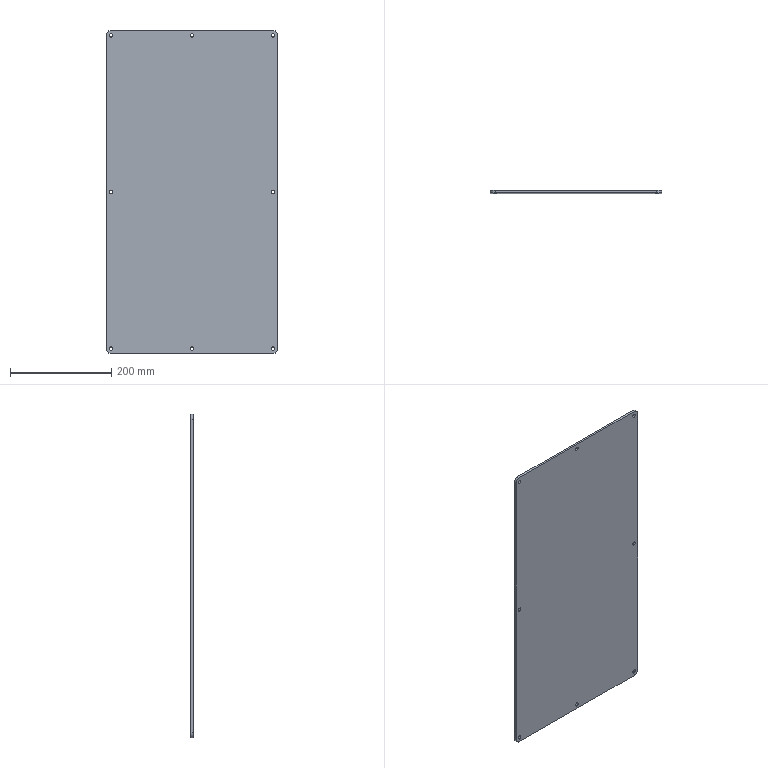Part | STEP file | b-006 | 1 solid | 26 faces | box 340 x 5 x 640 mm | volume 1086031 mm3 | cylinder 20 | plane 6 | commonest cylinder face diameters 7 x16 20 x4